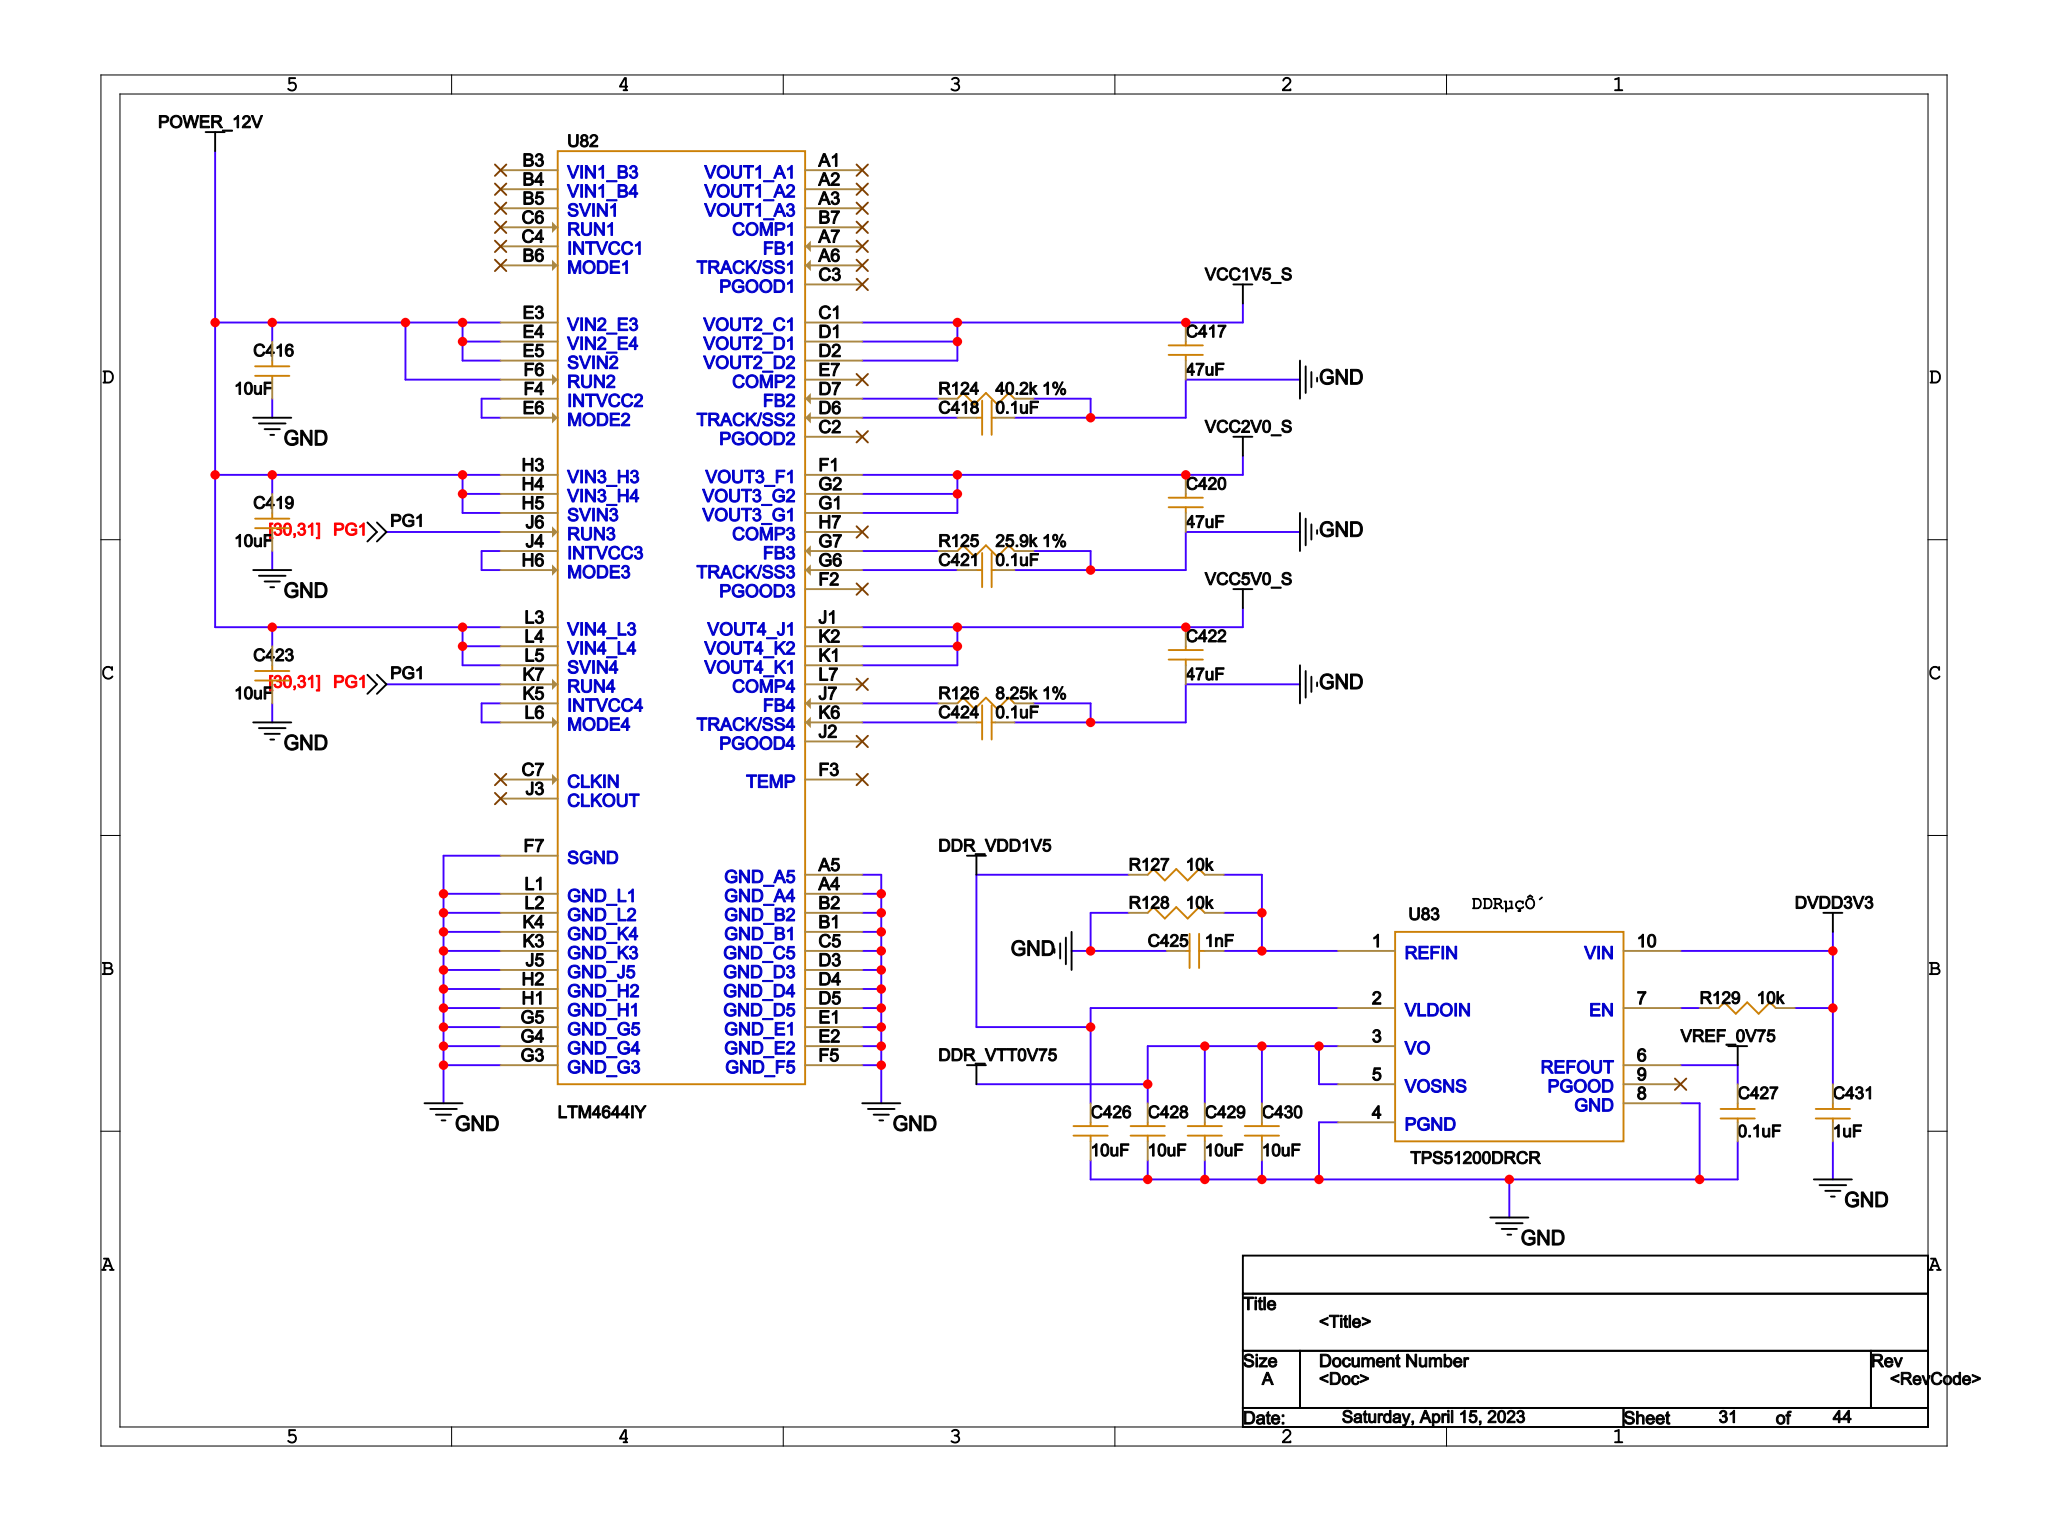Circuit board | Cadence Allegro | 1034 parts | 912 nets | one sheet of the schematic
Parts on this sheet (reference | value | footprint):
C416 | 10uF | C0402
C417 | 47uF | C0402
C418 | 0.1uF | C0402
C419 | 10uF | C0402
C420 | 47uF | C0402
C421 | 0.1uF | C0402
C422 | 47uF | C0402
C423 | 10uF | C0402
C424 | 0.1uF | C0402
C425 | 1nF | C0402
C426 | 10uF | C0402
C427 | 0.1uF | C0402
C428 | 10uF | C0402
C429 | 10uF | C0402
C430 | 10uF | C0402
C431 | 1uF | C0402
R124 | 40.2k 1% | R0402
R125 | 25.9k 1% | R0402
R126 | 8.25k 1% | R0402
R127 | 10k | R0402
R128 | 10k | R0402
R129 | 10k | R0402
U82 | LTM4644IY | BGA77-1_27-15_0X9_0-H5_21
U83 | TPS51200DRCR | SON10_TPS51200
Nets of these parts (net: part-pin ...):
GND: C416-1 C417-2 C418-1 C419-1 C420-2 C421-1 C422-2 C423-1 C424-1 C425-1 C426-2 C427-1 C428-2 C429-2 C430-2 C431-1 R124-2 R125-2 R126-2 R128-1 U83-4 U83-8 U82-A4 U82-A5 U82-B1 U82-B2 U82-C5 U82-D3 U82-D4 U82-D5 U82-E1 U82-E2 U82-F5 U82-F7 U82-G3 U82-G4 U82-G5 U82-H1 U82-H2 U82-J5 U82-K3 U82-K4 U82-L1 U82-L2
VREF_0V75: C427-2 U83-6
VCC5V0_S: C422-1 U82-J1 U82-K1 U82-K2
DDR_VTT0V75: C428-1 C429-1 C430-1 U83-3 U83-5
N13640051: R129-1 U83-7
N13638029: C425-2 R127-2 R128-2 U83-1
DVDD3V3: C431-2 R129-2 U83-10
DDR_VDD1V5: C426-1 R127-1 U83-2
N14057268: C418-2 U82-D6
N14058056: C421-2 U82-G6
N14116072: C424-2 U82-K6
VCC1V5_S: C417-1 U82-C1 U82-D1 U82-D2
VCC2V0_S: C420-1 U82-F1 U82-G1 U82-G2
POWER_12V: C416-2 C419-2 C423-2 U82-E3 U82-E4 U82-E5 U82-F6 U82-H3 U82-H4 U82-H5 U82-L3 U82-L4 U82-L5
PG1: U82-J6 U82-K7
N14057240: R124-1 U82-D7
N14058028: R125-1 U82-G7
N14116044: R126-1 U82-J7